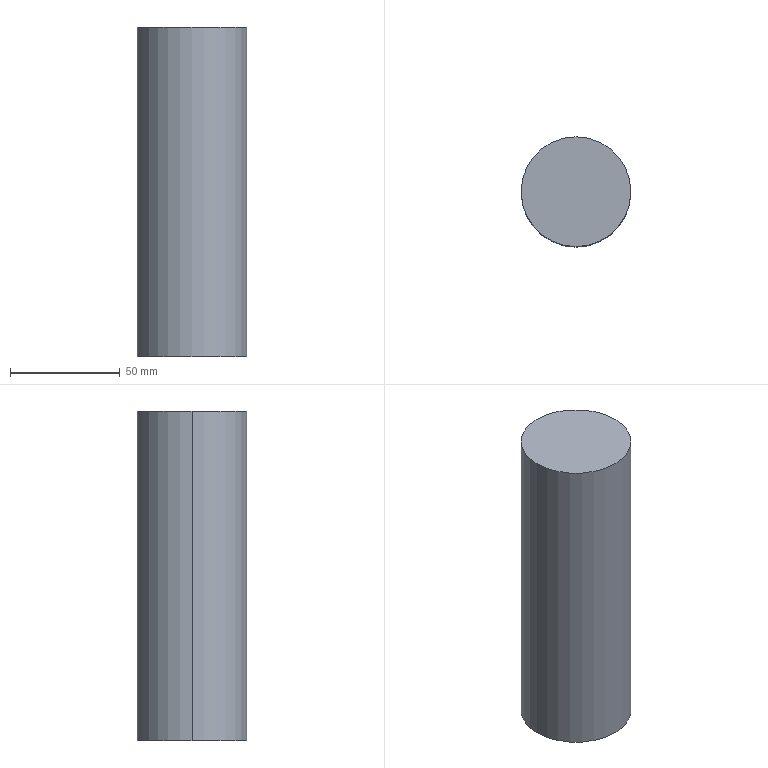Part | Creo | 1 solid | 8 faces | box 50 x 50 x 150 mm | volume 293732 mm3 | cylinder 4 | plane 2 | cone 2 | commonest cylinder face diameters 8 x2 50 x2
STEP:
#1=CARTESIAN_POINT('',(-30.,80.,-150.5));
#2=VERTEX_POINT('',#1);
#3=CARTESIAN_POINT('',(-80.,80.,-150.5));
#4=VERTEX_POINT('',#3);
#5=CARTESIAN_POINT('',(-55.,80.,-150.5));
#6=DIRECTION('',(0.,0.,1.));
#7=DIRECTION('',(1.,0.,0.));
#8=AXIS2_PLACEMENT_3D('',#5,#6,#7);
#9=CIRCLE('',#8,25.);
#10=EDGE_CURVE('',#2,#4,#9,.T.);
#11=ORIENTED_EDGE('',*,*,#10,.F.);
#12=CARTESIAN_POINT('',(-55.,80.,-150.5));
#13=DIRECTION('',(0.,0.,1.));
#14=DIRECTION('',(-1.,0.,0.));
#15=AXIS2_PLACEMENT_3D('',#12,#13,#14);
#16=CIRCLE('',#15,25.);
#17=EDGE_CURVE('',#4,#2,#16,.T.);
#18=ORIENTED_EDGE('',*,*,#17,.F.);
#19=EDGE_LOOP('',(#11,#18));
#20=FACE_OUTER_BOUND('',#19,.F.);
#21=CARTESIAN_POINT('',(-55.,80.,-150.5));
#22=DIRECTION('',(0.,0.,1.));
#23=DIRECTION('',(1.,0.,0.));
#24=AXIS2_PLACEMENT_3D('',#21,#22,#23);
#25=PLANE('',#24);
#26=ADVANCED_FACE('',(#20),#25,.T.);
#27=CARTESIAN_POINT('',(-80.,80.,-300.5));
#28=VERTEX_POINT('',#27);
#29=CARTESIAN_POINT('',(-30.,80.,-300.5));
#30=VERTEX_POINT('',#29);
#31=CARTESIAN_POINT('',(-55.,80.,-300.5));
#32=DIRECTION('',(0.,0.,-1.));
#33=DIRECTION('',(-1.,0.,0.));
#34=AXIS2_PLACEMENT_3D('',#31,#32,#33);
#35=CIRCLE('',#34,25.);
#36=EDGE_CURVE('',#28,#30,#35,.T.);
#37=ORIENTED_EDGE('',*,*,#36,.T.);
#38=CARTESIAN_POINT('',(-30.,80.,-150.5));
#39=DIRECTION('',(0.,0.,-1.));
#40=VECTOR('',#39,150.);
#41=LINE('',#38,#40);
#42=EDGE_CURVE('',#2,#30,#41,.T.);
#43=ORIENTED_EDGE('',*,*,#42,.F.);
#44=ORIENTED_EDGE('',*,*,#10,.T.);
#45=CARTESIAN_POINT('',(-80.,80.,-150.5));
#46=DIRECTION('',(0.,0.,-1.));
#47=VECTOR('',#46,150.);
#48=LINE('',#45,#47);
#49=EDGE_CURVE('',#4,#28,#48,.T.);
#50=ORIENTED_EDGE('',*,*,#49,.T.);
#51=EDGE_LOOP('',(#37,#43,#44,#50));
#52=FACE_OUTER_BOUND('',#51,.F.);
#53=CARTESIAN_POINT('',(-55.,80.,-150.5));
#54=DIRECTION('',(0.,0.,-1.));
#55=DIRECTION('',(-1.,0.,0.));
#56=AXIS2_PLACEMENT_3D('',#53,#54,#55);
#57=CYLINDRICAL_SURFACE('',#56,25.);
#58=ADVANCED_FACE('',(#52),#57,.T.);
#59=ORIENTED_EDGE('',*,*,#36,.F.);
#60=CARTESIAN_POINT('',(-55.,80.,-300.5));
#61=DIRECTION('',(0.,0.,-1.));
#62=DIRECTION('',(1.,0.,0.));
#63=AXIS2_PLACEMENT_3D('',#60,#61,#62);
#64=CIRCLE('',#63,25.);
#65=EDGE_CURVE('',#30,#28,#64,.T.);
#66=ORIENTED_EDGE('',*,*,#65,.F.);
#67=EDGE_LOOP('',(#59,#66));
#68=FACE_OUTER_BOUND('',#67,.F.);
#69=CARTESIAN_POINT('',(-51.,80.,-300.5));
#70=VERTEX_POINT('',#69);
#71=CARTESIAN_POINT('',(-59.,80.,-300.5));
#72=VERTEX_POINT('',#71);
#73=CARTESIAN_POINT('',(-55.,80.,-300.5));
#74=DIRECTION('',(0.,0.,1.));
#75=DIRECTION('',(1.,0.,0.));
#76=AXIS2_PLACEMENT_3D('',#73,#74,#75);
#77=CIRCLE('',#76,4.);
#78=EDGE_CURVE('',#70,#72,#77,.T.);
#79=ORIENTED_EDGE('',*,*,#78,.F.);
#80=CARTESIAN_POINT('',(-55.,80.,-300.5));
#81=DIRECTION('',(0.,0.,1.));
#82=DIRECTION('',(-1.,0.,0.));
#83=AXIS2_PLACEMENT_3D('',#80,#81,#82);
#84=CIRCLE('',#83,4.);
#85=EDGE_CURVE('',#72,#70,#84,.T.);
#86=ORIENTED_EDGE('',*,*,#85,.F.);
#87=EDGE_LOOP('',(#79,#86));
#88=FACE_BOUND('',#87,.F.);
#89=CARTESIAN_POINT('',(-55.,80.,-300.5));
#90=DIRECTION('',(0.,0.,-1.));
#91=DIRECTION('',(-1.,0.,0.));
#92=AXIS2_PLACEMENT_3D('',#89,#90,#91);
#93=PLANE('',#92);
#94=ADVANCED_FACE('',(#68,#88),#93,.T.);
#95=CARTESIAN_POINT('',(-59.,80.,-285.5));
#96=VERTEX_POINT('',#95);
#97=CARTESIAN_POINT('',(-51.,80.,-285.5));
#98=VERTEX_POINT('',#97);
#99=CARTESIAN_POINT('',(-55.,80.,-285.5));
#100=DIRECTION('',(0.,0.,-1.));
#101=DIRECTION('',(-1.,0.,0.));
#102=AXIS2_PLACEMENT_3D('',#99,#100,#101);
#103=CIRCLE('',#102,4.);
#104=EDGE_CURVE('',#96,#98,#103,.T.);
#105=ORIENTED_EDGE('',*,*,#104,.T.);
#106=CARTESIAN_POINT('',(-51.,80.,-300.5));
#107=DIRECTION('',(0.,0.,1.));
#108=VECTOR('',#107,15.);
#109=LINE('',#106,#108);
#110=EDGE_CURVE('',#70,#98,#109,.T.);
#111=ORIENTED_EDGE('',*,*,#110,.F.);
#112=ORIENTED_EDGE('',*,*,#78,.T.);
#113=CARTESIAN_POINT('',(-59.,80.,-300.5));
#114=DIRECTION('',(0.,0.,1.));
#115=VECTOR('',#114,15.);
#116=LINE('',#113,#115);
#117=EDGE_CURVE('',#72,#96,#116,.T.);
#118=ORIENTED_EDGE('',*,*,#117,.T.);
#119=EDGE_LOOP('',(#105,#111,#112,#118));
#120=FACE_OUTER_BOUND('',#119,.F.);
#121=CARTESIAN_POINT('',(-55.,80.,-300.5));
#122=DIRECTION('',(0.,0.,1.));
#123=DIRECTION('',(1.,0.,0.));
#124=AXIS2_PLACEMENT_3D('',#121,#122,#123);
#125=CYLINDRICAL_SURFACE('',#124,4.);
#126=ADVANCED_FACE('',(#120),#125,.F.);
#127=ORIENTED_EDGE('',*,*,#104,.F.);
#128=CARTESIAN_POINT('',(-55.,80.,-283.19));
#129=VERTEX_POINT('',#128);
#130=CARTESIAN_POINT('',(-55.,80.,-283.19));
#131=DIRECTION('',(-0.866,0.,-0.5001));
#132=VECTOR('',#131,4.619);
#133=LINE('',#130,#132);
#134=EDGE_CURVE('',#129,#96,#133,.T.);
#135=ORIENTED_EDGE('',*,*,#134,.F.);
#136=CARTESIAN_POINT('',(-55.,80.,-283.19));
#137=DIRECTION('',(0.866,0.,-0.5001));
#138=VECTOR('',#137,4.619);
#139=LINE('',#136,#138);
#140=EDGE_CURVE('',#129,#98,#139,.T.);
#141=ORIENTED_EDGE('',*,*,#140,.T.);
#142=EDGE_LOOP('',(#127,#135,#141));
#143=FACE_OUTER_BOUND('',#142,.F.);
#144=CARTESIAN_POINT('',(-55.,80.,-284.395));
#145=DIRECTION('',(0.,0.,-1.));
#146=DIRECTION('',(-1.,0.,0.));
#147=AXIS2_PLACEMENT_3D('',#144,#145,#146);
#148=CONICAL_SURFACE('',#147,2.086,59.994);
#149=ADVANCED_FACE('',(#143),#148,.F.);
#150=CARTESIAN_POINT('',(-55.,80.,-285.5));
#151=DIRECTION('',(0.,0.,-1.));
#152=DIRECTION('',(1.,0.,0.));
#153=AXIS2_PLACEMENT_3D('',#150,#151,#152);
#154=CIRCLE('',#153,4.);
#155=EDGE_CURVE('',#98,#96,#154,.T.);
#156=ORIENTED_EDGE('',*,*,#155,.F.);
#157=ORIENTED_EDGE('',*,*,#140,.F.);
#158=ORIENTED_EDGE('',*,*,#134,.T.);
#159=EDGE_LOOP('',(#156,#157,#158));
#160=FACE_OUTER_BOUND('',#159,.F.);
#161=CARTESIAN_POINT('',(-55.,80.,-284.395));
#162=DIRECTION('',(0.,0.,-1.));
#163=DIRECTION('',(-1.,0.,0.));
#164=AXIS2_PLACEMENT_3D('',#161,#162,#163);
#165=CONICAL_SURFACE('',#164,2.086,59.994);
#166=ADVANCED_FACE('',(#160),#165,.F.);
#167=ORIENTED_EDGE('',*,*,#155,.T.);
#168=ORIENTED_EDGE('',*,*,#117,.F.);
#169=ORIENTED_EDGE('',*,*,#85,.T.);
#170=ORIENTED_EDGE('',*,*,#110,.T.);
#171=EDGE_LOOP('',(#167,#168,#169,#170));
#172=FACE_OUTER_BOUND('',#171,.F.);
#173=CARTESIAN_POINT('',(-55.,80.,-300.5));
#174=DIRECTION('',(0.,0.,1.));
#175=DIRECTION('',(1.,0.,0.));
#176=AXIS2_PLACEMENT_3D('',#173,#174,#175);
#177=CYLINDRICAL_SURFACE('',#176,4.);
#178=ADVANCED_FACE('',(#172),#177,.F.);
#179=ORIENTED_EDGE('',*,*,#65,.T.);
#180=ORIENTED_EDGE('',*,*,#49,.F.);
#181=ORIENTED_EDGE('',*,*,#17,.T.);
#182=ORIENTED_EDGE('',*,*,#42,.T.);
#183=EDGE_LOOP('',(#179,#180,#181,#182));
#184=FACE_OUTER_BOUND('',#183,.F.);
#185=CARTESIAN_POINT('',(-55.,80.,-150.5));
#186=DIRECTION('',(0.,0.,-1.));
#187=DIRECTION('',(-1.,0.,0.));
#188=AXIS2_PLACEMENT_3D('',#185,#186,#187);
#189=CYLINDRICAL_SURFACE('',#188,25.);
#190=ADVANCED_FACE('',(#184),#189,.T.);
#191=CLOSED_SHELL('',(#26,#58,#94,#126,#149,#166,#178,#190));
#192=MANIFOLD_SOLID_BREP('',#191);
#193=(LENGTH_UNIT()NAMED_UNIT(*)SI_UNIT(.MILLI.,.METRE.));
#194=UNCERTAINTY_MEASURE_WITH_UNIT(LENGTH_MEASURE(0.01658),#193,'','');
#195=(NAMED_UNIT(*)PLANE_ANGLE_UNIT()SI_UNIT($,.RADIAN.));
#196=PLANE_ANGLE_MEASURE_WITH_UNIT(PLANE_ANGLE_MEASURE(0.01745),#195);
#197=(CONVERSION_BASED_UNIT('DEGREE',#196)NAMED_UNIT(*)PLANE_ANGLE_UNIT());
#198=(NAMED_UNIT(*)SI_UNIT($,.STERADIAN.)SOLID_ANGLE_UNIT());
#199=(GEOMETRIC_REPRESENTATION_CONTEXT(3)GLOBAL_UNCERTAINTY_ASSIGNED_CONTEXT((#194))GLOBAL_UNIT_ASSIGNED_CONTEXT((#193,#197,#198))REPRESENTATION_CONTEXT('',''));
#200=ADVANCED_BREP_SHAPE_REPRESENTATION('',(#192),#199);